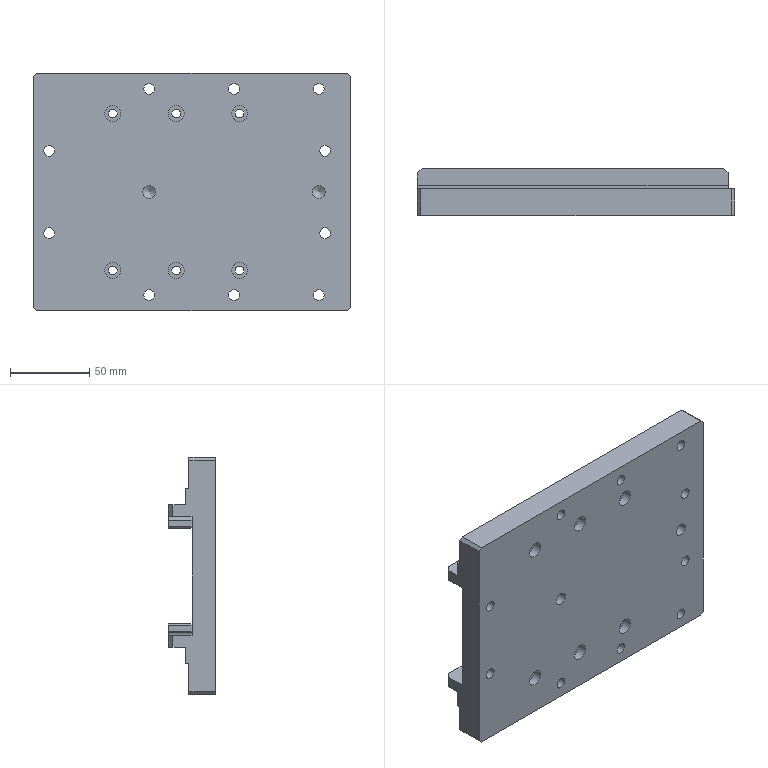Part | 1 solid | 85 faces | box 200 x 30 x 150 mm | volume 547054 mm3 | plane 45 | cylinder 33 | cone 7 | commonest cylinder face diameters 6.8 x10 5.5 x6 10 x6 5 x4 4.2 x3 2.5 x2